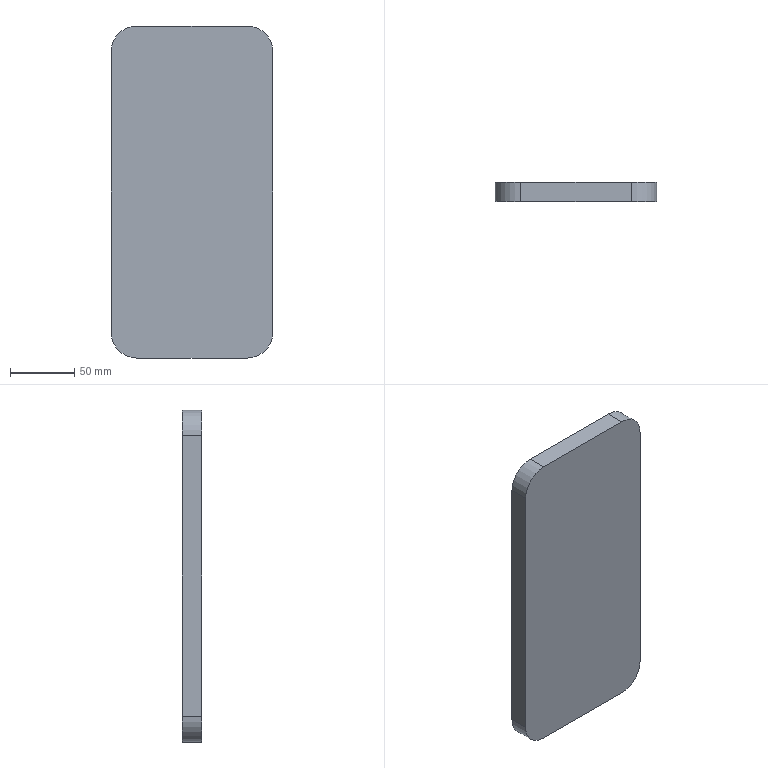Part | SolidWorks | features DeleteBody 1, MBimport 1 | 1 solid | 10 faces | box 126 x 15 x 258.5 mm | volume 483415 mm3 | plane 6 | cylinder 4 | commonest cylinder face diameters 40 x4
STEP:
#1=CARTESIAN_POINT('',(111.,-393.,-1386.5));
#2=VERTEX_POINT('',#1);
#3=CARTESIAN_POINT('',(111.,-393.,-1605.));
#4=VERTEX_POINT('',#3);
#5=CARTESIAN_POINT('',(111.,-393.,-1386.5));
#6=DIRECTION('',(0.,0.,-1.));
#7=VECTOR('',#6,1000.);
#8=LINE('',#5,#7);
#9=EDGE_CURVE('',#2,#4,#8,.T.);
#10=ORIENTED_EDGE('',*,*,#9,.F.);
#11=CARTESIAN_POINT('',(131.,-393.,-1366.5));
#12=VERTEX_POINT('',#11);
#13=CARTESIAN_POINT('',(131.,-393.,-1386.5));
#14=DIRECTION('',(0.,-1.,0.));
#15=DIRECTION('',(1.,0.,0.));
#16=AXIS2_PLACEMENT_3D('',#13,#14,#15);
#17=CIRCLE('',#16,20.);
#18=EDGE_CURVE('',#12,#2,#17,.T.);
#19=ORIENTED_EDGE('',*,*,#18,.F.);
#20=CARTESIAN_POINT('',(217.,-393.,-1366.5));
#21=VERTEX_POINT('',#20);
#22=CARTESIAN_POINT('',(217.,-393.,-1366.5));
#23=DIRECTION('',(-1.,0.,0.));
#24=VECTOR('',#23,1000.);
#25=LINE('',#22,#24);
#26=EDGE_CURVE('',#21,#12,#25,.T.);
#27=ORIENTED_EDGE('',*,*,#26,.F.);
#28=CARTESIAN_POINT('',(237.,-393.,-1386.5));
#29=VERTEX_POINT('',#28);
#30=CARTESIAN_POINT('',(217.,-393.,-1386.5));
#31=DIRECTION('',(0.,-1.,0.));
#32=DIRECTION('',(1.,0.,0.));
#33=AXIS2_PLACEMENT_3D('',#30,#31,#32);
#34=CIRCLE('',#33,20.);
#35=EDGE_CURVE('',#29,#21,#34,.T.);
#36=ORIENTED_EDGE('',*,*,#35,.F.);
#37=CARTESIAN_POINT('',(237.,-393.,-1605.));
#38=VERTEX_POINT('',#37);
#39=CARTESIAN_POINT('',(237.,-393.,-1605.));
#40=DIRECTION('',(0.,0.,1.));
#41=VECTOR('',#40,1000.);
#42=LINE('',#39,#41);
#43=EDGE_CURVE('',#38,#29,#42,.T.);
#44=ORIENTED_EDGE('',*,*,#43,.F.);
#45=CARTESIAN_POINT('',(217.,-393.,-1625.));
#46=VERTEX_POINT('',#45);
#47=CARTESIAN_POINT('',(217.,-393.,-1605.));
#48=DIRECTION('',(0.,-1.,0.));
#49=DIRECTION('',(1.,0.,0.));
#50=AXIS2_PLACEMENT_3D('',#47,#48,#49);
#51=CIRCLE('',#50,20.);
#52=EDGE_CURVE('',#46,#38,#51,.T.);
#53=ORIENTED_EDGE('',*,*,#52,.F.);
#54=CARTESIAN_POINT('',(131.,-393.,-1625.));
#55=VERTEX_POINT('',#54);
#56=CARTESIAN_POINT('',(131.,-393.,-1625.));
#57=DIRECTION('',(1.,0.,0.));
#58=VECTOR('',#57,1000.);
#59=LINE('',#56,#58);
#60=EDGE_CURVE('',#55,#46,#59,.T.);
#61=ORIENTED_EDGE('',*,*,#60,.F.);
#62=CARTESIAN_POINT('',(131.,-393.,-1605.));
#63=DIRECTION('',(0.,-1.,0.));
#64=DIRECTION('',(1.,0.,0.));
#65=AXIS2_PLACEMENT_3D('',#62,#63,#64);
#66=CIRCLE('',#65,20.);
#67=EDGE_CURVE('',#4,#55,#66,.T.);
#68=ORIENTED_EDGE('',*,*,#67,.F.);
#69=EDGE_LOOP('',(#10,#19,#27,#36,#44,#53,#61,#68));
#70=FACE_OUTER_BOUND('',#69,.T.);
#71=CARTESIAN_POINT('',(131.,-393.,-1605.));
#72=DIRECTION('',(0.,-1.,0.));
#73=DIRECTION('',(0.,0.,-1.));
#74=AXIS2_PLACEMENT_3D('',#71,#72,#73);
#75=PLANE('',#74);
#76=ADVANCED_FACE('',(#70),#75,.F.);
#77=CARTESIAN_POINT('',(111.,-408.,-1386.5));
#78=VERTEX_POINT('',#77);
#79=CARTESIAN_POINT('',(111.,-408.,-1605.));
#80=VERTEX_POINT('',#79);
#81=CARTESIAN_POINT('',(111.,-408.,-1386.5));
#82=DIRECTION('',(0.,0.,-1.));
#83=VECTOR('',#82,1000.);
#84=LINE('',#81,#83);
#85=EDGE_CURVE('',#78,#80,#84,.T.);
#86=ORIENTED_EDGE('',*,*,#85,.T.);
#87=CARTESIAN_POINT('',(131.,-408.,-1625.));
#88=VERTEX_POINT('',#87);
#89=CARTESIAN_POINT('',(131.,-408.,-1605.));
#90=DIRECTION('',(0.,-1.,0.));
#91=DIRECTION('',(1.,0.,0.));
#92=AXIS2_PLACEMENT_3D('',#89,#90,#91);
#93=CIRCLE('',#92,20.);
#94=EDGE_CURVE('',#80,#88,#93,.T.);
#95=ORIENTED_EDGE('',*,*,#94,.T.);
#96=CARTESIAN_POINT('',(217.,-408.,-1625.));
#97=VERTEX_POINT('',#96);
#98=CARTESIAN_POINT('',(131.,-408.,-1625.));
#99=DIRECTION('',(1.,0.,0.));
#100=VECTOR('',#99,1000.);
#101=LINE('',#98,#100);
#102=EDGE_CURVE('',#88,#97,#101,.T.);
#103=ORIENTED_EDGE('',*,*,#102,.T.);
#104=CARTESIAN_POINT('',(237.,-408.,-1605.));
#105=VERTEX_POINT('',#104);
#106=CARTESIAN_POINT('',(217.,-408.,-1605.));
#107=DIRECTION('',(0.,-1.,0.));
#108=DIRECTION('',(1.,0.,0.));
#109=AXIS2_PLACEMENT_3D('',#106,#107,#108);
#110=CIRCLE('',#109,20.);
#111=EDGE_CURVE('',#97,#105,#110,.T.);
#112=ORIENTED_EDGE('',*,*,#111,.T.);
#113=CARTESIAN_POINT('',(237.,-408.,-1386.5));
#114=VERTEX_POINT('',#113);
#115=CARTESIAN_POINT('',(237.,-408.,-1605.));
#116=DIRECTION('',(0.,0.,1.));
#117=VECTOR('',#116,1000.);
#118=LINE('',#115,#117);
#119=EDGE_CURVE('',#105,#114,#118,.T.);
#120=ORIENTED_EDGE('',*,*,#119,.T.);
#121=CARTESIAN_POINT('',(217.,-408.,-1366.5));
#122=VERTEX_POINT('',#121);
#123=CARTESIAN_POINT('',(217.,-408.,-1386.5));
#124=DIRECTION('',(0.,-1.,0.));
#125=DIRECTION('',(1.,0.,0.));
#126=AXIS2_PLACEMENT_3D('',#123,#124,#125);
#127=CIRCLE('',#126,20.);
#128=EDGE_CURVE('',#114,#122,#127,.T.);
#129=ORIENTED_EDGE('',*,*,#128,.T.);
#130=CARTESIAN_POINT('',(131.,-408.,-1366.5));
#131=VERTEX_POINT('',#130);
#132=CARTESIAN_POINT('',(217.,-408.,-1366.5));
#133=DIRECTION('',(-1.,0.,0.));
#134=VECTOR('',#133,1000.);
#135=LINE('',#132,#134);
#136=EDGE_CURVE('',#122,#131,#135,.T.);
#137=ORIENTED_EDGE('',*,*,#136,.T.);
#138=CARTESIAN_POINT('',(131.,-408.,-1386.5));
#139=DIRECTION('',(0.,-1.,0.));
#140=DIRECTION('',(1.,0.,0.));
#141=AXIS2_PLACEMENT_3D('',#138,#139,#140);
#142=CIRCLE('',#141,20.);
#143=EDGE_CURVE('',#131,#78,#142,.T.);
#144=ORIENTED_EDGE('',*,*,#143,.T.);
#145=EDGE_LOOP('',(#86,#95,#103,#112,#120,#129,#137,#144));
#146=FACE_OUTER_BOUND('',#145,.T.);
#147=CARTESIAN_POINT('',(131.,-408.,-1605.));
#148=DIRECTION('',(0.,-1.,0.));
#149=DIRECTION('',(0.,0.,-1.));
#150=AXIS2_PLACEMENT_3D('',#147,#148,#149);
#151=PLANE('',#150);
#152=ADVANCED_FACE('',(#146),#151,.T.);
#153=ORIENTED_EDGE('',*,*,#18,.T.);
#154=CARTESIAN_POINT('',(111.,-408.,-1386.5));
#155=DIRECTION('',(0.,1.,0.));
#156=VECTOR('',#155,1000.);
#157=LINE('',#154,#156);
#158=EDGE_CURVE('',#78,#2,#157,.T.);
#159=ORIENTED_EDGE('',*,*,#158,.F.);
#160=ORIENTED_EDGE('',*,*,#143,.F.);
#161=CARTESIAN_POINT('',(131.,-408.,-1366.5));
#162=DIRECTION('',(0.,1.,0.));
#163=VECTOR('',#162,1000.);
#164=LINE('',#161,#163);
#165=EDGE_CURVE('',#131,#12,#164,.T.);
#166=ORIENTED_EDGE('',*,*,#165,.T.);
#167=EDGE_LOOP('',(#153,#159,#160,#166));
#168=FACE_OUTER_BOUND('',#167,.T.);
#169=CARTESIAN_POINT('',(131.,-408.,-1386.5));
#170=DIRECTION('',(0.,1.,0.));
#171=DIRECTION('',(0.,0.,1.));
#172=AXIS2_PLACEMENT_3D('',#169,#170,#171);
#173=CYLINDRICAL_SURFACE('',#172,20.);
#174=ADVANCED_FACE('',(#168),#173,.T.);
#175=ORIENTED_EDGE('',*,*,#26,.T.);
#176=ORIENTED_EDGE('',*,*,#165,.F.);
#177=ORIENTED_EDGE('',*,*,#136,.F.);
#178=CARTESIAN_POINT('',(217.,-408.,-1366.5));
#179=DIRECTION('',(0.,1.,0.));
#180=VECTOR('',#179,1000.);
#181=LINE('',#178,#180);
#182=EDGE_CURVE('',#122,#21,#181,.T.);
#183=ORIENTED_EDGE('',*,*,#182,.T.);
#184=EDGE_LOOP('',(#175,#176,#177,#183));
#185=FACE_OUTER_BOUND('',#184,.T.);
#186=CARTESIAN_POINT('',(217.,-408.,-1366.5));
#187=DIRECTION('',(0.,0.,-1.));
#188=DIRECTION('',(-1.,0.,0.));
#189=AXIS2_PLACEMENT_3D('',#186,#187,#188);
#190=PLANE('',#189);
#191=ADVANCED_FACE('',(#185),#190,.F.);
#192=ORIENTED_EDGE('',*,*,#35,.T.);
#193=ORIENTED_EDGE('',*,*,#182,.F.);
#194=ORIENTED_EDGE('',*,*,#128,.F.);
#195=CARTESIAN_POINT('',(237.,-408.,-1386.5));
#196=DIRECTION('',(0.,1.,0.));
#197=VECTOR('',#196,1000.);
#198=LINE('',#195,#197);
#199=EDGE_CURVE('',#114,#29,#198,.T.);
#200=ORIENTED_EDGE('',*,*,#199,.T.);
#201=EDGE_LOOP('',(#192,#193,#194,#200));
#202=FACE_OUTER_BOUND('',#201,.T.);
#203=CARTESIAN_POINT('',(217.,-408.,-1386.5));
#204=DIRECTION('',(0.,1.,0.));
#205=DIRECTION('',(0.,0.,1.));
#206=AXIS2_PLACEMENT_3D('',#203,#204,#205);
#207=CYLINDRICAL_SURFACE('',#206,20.);
#208=ADVANCED_FACE('',(#202),#207,.T.);
#209=ORIENTED_EDGE('',*,*,#43,.T.);
#210=ORIENTED_EDGE('',*,*,#199,.F.);
#211=ORIENTED_EDGE('',*,*,#119,.F.);
#212=CARTESIAN_POINT('',(237.,-408.,-1605.));
#213=DIRECTION('',(0.,1.,0.));
#214=VECTOR('',#213,1000.);
#215=LINE('',#212,#214);
#216=EDGE_CURVE('',#105,#38,#215,.T.);
#217=ORIENTED_EDGE('',*,*,#216,.T.);
#218=EDGE_LOOP('',(#209,#210,#211,#217));
#219=FACE_OUTER_BOUND('',#218,.T.);
#220=CARTESIAN_POINT('',(237.,-408.,-1605.));
#221=DIRECTION('',(-1.,0.,0.));
#222=DIRECTION('',(0.,1.,0.));
#223=AXIS2_PLACEMENT_3D('',#220,#221,#222);
#224=PLANE('',#223);
#225=ADVANCED_FACE('',(#219),#224,.F.);
#226=ORIENTED_EDGE('',*,*,#52,.T.);
#227=ORIENTED_EDGE('',*,*,#216,.F.);
#228=ORIENTED_EDGE('',*,*,#111,.F.);
#229=CARTESIAN_POINT('',(217.,-408.,-1625.));
#230=DIRECTION('',(0.,1.,0.));
#231=VECTOR('',#230,1000.);
#232=LINE('',#229,#231);
#233=EDGE_CURVE('',#97,#46,#232,.T.);
#234=ORIENTED_EDGE('',*,*,#233,.T.);
#235=EDGE_LOOP('',(#226,#227,#228,#234));
#236=FACE_OUTER_BOUND('',#235,.T.);
#237=CARTESIAN_POINT('',(217.,-408.,-1605.));
#238=DIRECTION('',(0.,1.,0.));
#239=DIRECTION('',(0.,0.,1.));
#240=AXIS2_PLACEMENT_3D('',#237,#238,#239);
#241=CYLINDRICAL_SURFACE('',#240,20.);
#242=ADVANCED_FACE('',(#236),#241,.T.);
#243=ORIENTED_EDGE('',*,*,#60,.T.);
#244=ORIENTED_EDGE('',*,*,#233,.F.);
#245=ORIENTED_EDGE('',*,*,#102,.F.);
#246=CARTESIAN_POINT('',(131.,-408.,-1625.));
#247=DIRECTION('',(0.,1.,0.));
#248=VECTOR('',#247,1000.);
#249=LINE('',#246,#248);
#250=EDGE_CURVE('',#88,#55,#249,.T.);
#251=ORIENTED_EDGE('',*,*,#250,.T.);
#252=EDGE_LOOP('',(#243,#244,#245,#251));
#253=FACE_OUTER_BOUND('',#252,.T.);
#254=CARTESIAN_POINT('',(131.,-408.,-1625.));
#255=DIRECTION('',(0.,0.,1.));
#256=DIRECTION('',(1.,0.,0.));
#257=AXIS2_PLACEMENT_3D('',#254,#255,#256);
#258=PLANE('',#257);
#259=ADVANCED_FACE('',(#253),#258,.F.);
#260=ORIENTED_EDGE('',*,*,#67,.T.);
#261=ORIENTED_EDGE('',*,*,#250,.F.);
#262=ORIENTED_EDGE('',*,*,#94,.F.);
#263=CARTESIAN_POINT('',(111.,-408.,-1605.));
#264=DIRECTION('',(0.,1.,0.));
#265=VECTOR('',#264,1000.);
#266=LINE('',#263,#265);
#267=EDGE_CURVE('',#80,#4,#266,.T.);
#268=ORIENTED_EDGE('',*,*,#267,.T.);
#269=EDGE_LOOP('',(#260,#261,#262,#268));
#270=FACE_OUTER_BOUND('',#269,.T.);
#271=CARTESIAN_POINT('',(131.,-408.,-1605.));
#272=DIRECTION('',(0.,1.,0.));
#273=DIRECTION('',(0.,0.,1.));
#274=AXIS2_PLACEMENT_3D('',#271,#272,#273);
#275=CYLINDRICAL_SURFACE('',#274,20.);
#276=ADVANCED_FACE('',(#270),#275,.T.);
#277=ORIENTED_EDGE('',*,*,#9,.T.);
#278=ORIENTED_EDGE('',*,*,#267,.F.);
#279=ORIENTED_EDGE('',*,*,#85,.F.);
#280=ORIENTED_EDGE('',*,*,#158,.T.);
#281=EDGE_LOOP('',(#277,#278,#279,#280));
#282=FACE_OUTER_BOUND('',#281,.T.);
#283=CARTESIAN_POINT('',(111.,-408.,-1386.5));
#284=DIRECTION('',(1.,0.,0.));
#285=DIRECTION('',(0.,0.,-1.));
#286=AXIS2_PLACEMENT_3D('',#283,#284,#285);
#287=PLANE('',#286);
#288=ADVANCED_FACE('',(#282),#287,.F.);
#289=CLOSED_SHELL('',(#76,#152,#174,#191,#208,#225,#242,#259,#276,#288));
#290=MANIFOLD_SOLID_BREP('',#289);
#291=CARTESIAN_POINT('',(0.,0.,0.));
#292=DIRECTION('',(0.,0.,1.));
#293=DIRECTION('',(1.,0.,0.));
#294=AXIS2_PLACEMENT_3D('',#291,#292,#293);
#295=(LENGTH_UNIT()NAMED_UNIT(*)SI_UNIT(.MILLI.,.METRE.));
#296=UNCERTAINTY_MEASURE_WITH_UNIT(LENGTH_MEASURE(0.00001),#295,'','');
#297=(NAMED_UNIT(*)PLANE_ANGLE_UNIT()SI_UNIT($,.RADIAN.));
#298=(NAMED_UNIT(*)SI_UNIT($,.STERADIAN.)SOLID_ANGLE_UNIT());
#299=(GEOMETRIC_REPRESENTATION_CONTEXT(3)GLOBAL_UNCERTAINTY_ASSIGNED_CONTEXT((#296))GLOBAL_UNIT_ASSIGNED_CONTEXT((#295,#297,#298))REPRESENTATION_CONTEXT('',''));
#300=ADVANCED_BREP_SHAPE_REPRESENTATION('',(#290,#294),#299);